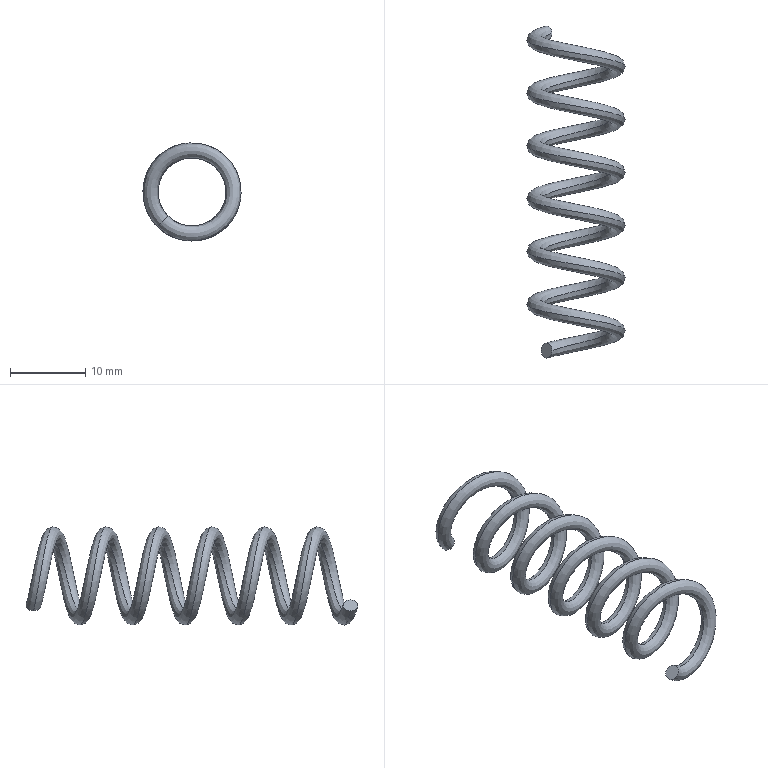Part | STEP file | Ngam kep 19 | 1 solid | 4 faces | box 13 x 44 x 13 mm | volume 652.249 mm3 | spline 2 | plane 2